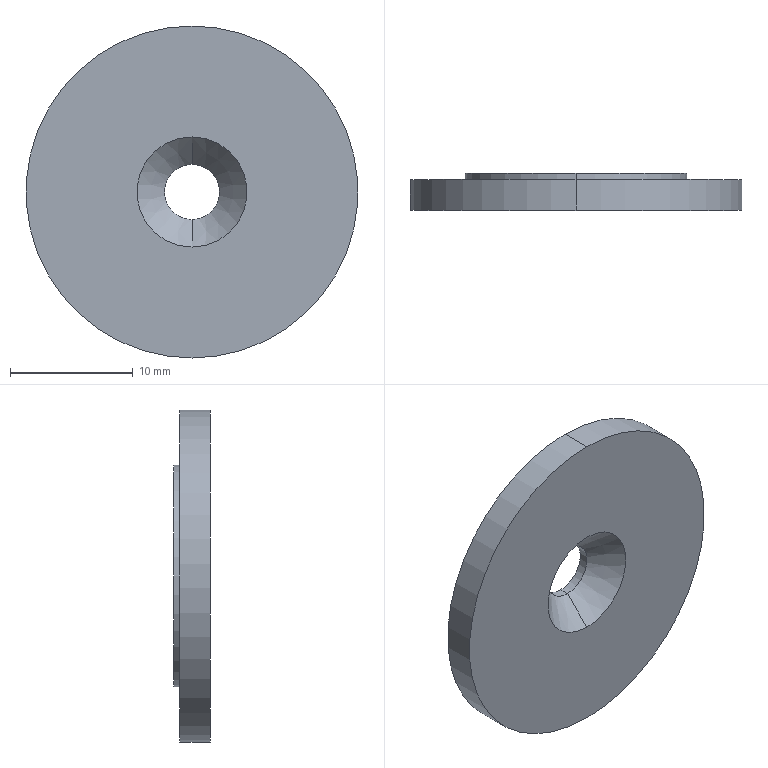Part | STEP file | ND25021-01-JDKM-14-TL | 1 solid | 11 faces | box 27 x 3 x 27 mm | volume 1464 mm3 | cylinder 6 | plane 3 | cone 2 | commonest cylinder face diameters 4.5 x2 18 x2 27 x2
STEP:
#1=CARTESIAN_POINT('',(0.,0.,0.));
#2=DIRECTION('',(0.,0.,1.));
#3=DIRECTION('',(1.,0.,0.));
#4=AXIS2_PLACEMENT_3D('',#1,#2,#3);
#5=CARTESIAN_POINT('',(0.,2.23,-2.25));
#6=VERTEX_POINT('',#5);
#7=CARTESIAN_POINT('',(0.,0.,-4.48));
#8=VERTEX_POINT('',#7);
#9=CARTESIAN_POINT('',(0.,0.,-4.48));
#10=DIRECTION('',(0.,-0.7071,-0.7071));
#11=VECTOR('',#10,1.);
#12=LINE('',#9,#11);
#13=CARTESIAN_POINT('',(0.,0.,0.));
#14=DIRECTION('',(0.,-1.,0.));
#15=DIRECTION('',(0.,0.,-1.));
#16=AXIS2_PLACEMENT_3D('',#13,#14,#15);
#17=CONICAL_SURFACE('',#16,4.48,0.7854);
#18=CARTESIAN_POINT('',(6.283,0.));
#19=DIRECTION('',(0.,1.));
#20=VECTOR('',#19,1.);
#21=LINE('',#18,#20);
#22=(GEOMETRIC_REPRESENTATION_CONTEXT(2)PARAMETRIC_REPRESENTATION_CONTEXT()REPRESENTATION_CONTEXT('',''));
#23=DEFINITIONAL_REPRESENTATION('',(#21),#22);
#24=PCURVE('',#17,#23);
#25=CARTESIAN_POINT('',(0.,0.,0.));
#26=DIRECTION('',(0.,-1.,0.));
#27=DIRECTION('',(0.,0.,-1.));
#28=AXIS2_PLACEMENT_3D('',#25,#26,#27);
#29=CONICAL_SURFACE('',#28,4.48,0.7854);
#30=CARTESIAN_POINT('',(0.,0.));
#31=DIRECTION('',(0.,1.));
#32=VECTOR('',#31,1.);
#33=LINE('',#30,#32);
#34=(GEOMETRIC_REPRESENTATION_CONTEXT(2)PARAMETRIC_REPRESENTATION_CONTEXT()REPRESENTATION_CONTEXT('',''));
#35=DEFINITIONAL_REPRESENTATION('',(#33),#34);
#36=PCURVE('',#29,#35);
#37=SURFACE_CURVE('',#12,(#24,#36),.PCURVE_S1.);
#38=EDGE_CURVE('',#6,#8,#37,.T.);
#39=ORIENTED_EDGE('',*,*,#38,.T.);
#40=CARTESIAN_POINT('',(0.,0.,4.48));
#41=VERTEX_POINT('',#40);
#42=CARTESIAN_POINT('',(0.,0.,0.));
#43=DIRECTION('',(0.,-1.,0.));
#44=DIRECTION('',(0.,0.,-1.));
#45=AXIS2_PLACEMENT_3D('',#42,#43,#44);
#46=CIRCLE('',#45,4.48);
#47=CARTESIAN_POINT('',(0.,0.));
#48=DIRECTION('',(1.,0.));
#49=VECTOR('',#48,1.);
#50=LINE('',#47,#49);
#51=(GEOMETRIC_REPRESENTATION_CONTEXT(2)PARAMETRIC_REPRESENTATION_CONTEXT()REPRESENTATION_CONTEXT('',''));
#52=DEFINITIONAL_REPRESENTATION('',(#50),#51);
#53=PCURVE('',#17,#52);
#54=CARTESIAN_POINT('',(0.,0.,0.));
#55=DIRECTION('',(0.,1.,0.));
#56=DIRECTION('',(0.,0.,1.));
#57=AXIS2_PLACEMENT_3D('',#54,#55,#56);
#58=PLANE('',#57);
#59=CARTESIAN_POINT('',(-4.48,0.));
#60=CARTESIAN_POINT('',(-4.48,7.76));
#61=CARTESIAN_POINT('',(2.24,3.88));
#62=CARTESIAN_POINT('',(8.96,0.));
#63=CARTESIAN_POINT('',(2.24,-3.88));
#64=CARTESIAN_POINT('',(-4.48,-7.76));
#65=CARTESIAN_POINT('',(-4.48,0.));
#66=(BOUNDED_CURVE()B_SPLINE_CURVE(2,(#59,#60,#61,#62,#63,#64,#65),.UNSPECIFIED.,.T.,.F.)B_SPLINE_CURVE_WITH_KNOTS((1,2,2,2,2,1),(-2.094,0.,2.094,4.189,6.283,8.378),.UNSPECIFIED.)CURVE()GEOMETRIC_REPRESENTATION_ITEM()RATIONAL_B_SPLINE_CURVE((1.,0.5,1.,0.5,1.,0.5,1.))REPRESENTATION_ITEM(''));
#67=(GEOMETRIC_REPRESENTATION_CONTEXT(2)PARAMETRIC_REPRESENTATION_CONTEXT()REPRESENTATION_CONTEXT('',''));
#68=DEFINITIONAL_REPRESENTATION('',(#66),#67);
#69=PCURVE('',#58,#68);
#70=SURFACE_CURVE('',#46,(#53,#69),.PCURVE_S1.);
#71=EDGE_CURVE('',#41,#8,#70,.T.);
#72=ORIENTED_EDGE('',*,*,#71,.F.);
#73=CARTESIAN_POINT('',(0.,2.23,2.25));
#74=VERTEX_POINT('',#73);
#75=CARTESIAN_POINT('',(0.,0.,4.48));
#76=DIRECTION('',(0.,-0.7071,0.7071));
#77=VECTOR('',#76,1.);
#78=LINE('',#75,#77);
#79=CARTESIAN_POINT('',(3.142,0.));
#80=DIRECTION('',(0.,1.));
#81=VECTOR('',#80,1.);
#82=LINE('',#79,#81);
#83=(GEOMETRIC_REPRESENTATION_CONTEXT(2)PARAMETRIC_REPRESENTATION_CONTEXT()REPRESENTATION_CONTEXT('',''));
#84=DEFINITIONAL_REPRESENTATION('',(#82),#83);
#85=PCURVE('',#17,#84);
#86=CARTESIAN_POINT('',(3.142,0.));
#87=DIRECTION('',(0.,1.));
#88=VECTOR('',#87,1.);
#89=LINE('',#86,#88);
#90=(GEOMETRIC_REPRESENTATION_CONTEXT(2)PARAMETRIC_REPRESENTATION_CONTEXT()REPRESENTATION_CONTEXT('',''));
#91=DEFINITIONAL_REPRESENTATION('',(#89),#90);
#92=PCURVE('',#29,#91);
#93=SURFACE_CURVE('',#78,(#85,#92),.PCURVE_S1.);
#94=EDGE_CURVE('',#74,#41,#93,.T.);
#95=ORIENTED_EDGE('',*,*,#94,.F.);
#96=CARTESIAN_POINT('',(0.,2.23,0.));
#97=DIRECTION('',(0.,-1.,0.));
#98=DIRECTION('',(0.,0.,-1.));
#99=AXIS2_PLACEMENT_3D('',#96,#97,#98);
#100=CIRCLE('',#99,2.25);
#101=CARTESIAN_POINT('',(0.,-2.23));
#102=DIRECTION('',(1.,0.));
#103=VECTOR('',#102,1.);
#104=LINE('',#101,#103);
#105=(GEOMETRIC_REPRESENTATION_CONTEXT(2)PARAMETRIC_REPRESENTATION_CONTEXT()REPRESENTATION_CONTEXT('',''));
#106=DEFINITIONAL_REPRESENTATION('',(#104),#105);
#107=PCURVE('',#17,#106);
#108=CARTESIAN_POINT('',(0.,0.,0.));
#109=DIRECTION('',(0.,-1.,0.));
#110=DIRECTION('',(0.,0.,-1.));
#111=AXIS2_PLACEMENT_3D('',#108,#109,#110);
#112=CYLINDRICAL_SURFACE('',#111,2.25);
#113=CARTESIAN_POINT('',(0.,-2.23));
#114=DIRECTION('',(1.,0.));
#115=VECTOR('',#114,1.);
#116=LINE('',#113,#115);
#117=(GEOMETRIC_REPRESENTATION_CONTEXT(2)PARAMETRIC_REPRESENTATION_CONTEXT()REPRESENTATION_CONTEXT('',''));
#118=DEFINITIONAL_REPRESENTATION('',(#116),#117);
#119=PCURVE('',#112,#118);
#120=SURFACE_CURVE('',#100,(#107,#119),.PCURVE_S1.);
#121=EDGE_CURVE('',#74,#6,#120,.T.);
#122=ORIENTED_EDGE('',*,*,#121,.T.);
#123=EDGE_LOOP('',(#39,#72,#95,#122));
#124=FACE_BOUND('',#123,.F.);
#125=ADVANCED_FACE('',(#124),#17,.F.);
#126=CARTESIAN_POINT('',(0.,3.,-2.25));
#127=VERTEX_POINT('',#126);
#128=CARTESIAN_POINT('',(0.,0.,-2.25));
#129=DIRECTION('',(0.,-1.,0.));
#130=VECTOR('',#129,1.);
#131=LINE('',#128,#130);
#132=CARTESIAN_POINT('',(6.283,0.));
#133=DIRECTION('',(0.,1.));
#134=VECTOR('',#133,1.);
#135=LINE('',#132,#134);
#136=(GEOMETRIC_REPRESENTATION_CONTEXT(2)PARAMETRIC_REPRESENTATION_CONTEXT()REPRESENTATION_CONTEXT('',''));
#137=DEFINITIONAL_REPRESENTATION('',(#135),#136);
#138=PCURVE('',#112,#137);
#139=CARTESIAN_POINT('',(0.,0.,0.));
#140=DIRECTION('',(0.,-1.,0.));
#141=DIRECTION('',(0.,0.,-1.));
#142=AXIS2_PLACEMENT_3D('',#139,#140,#141);
#143=CYLINDRICAL_SURFACE('',#142,2.25);
#144=CARTESIAN_POINT('',(0.,0.));
#145=DIRECTION('',(0.,1.));
#146=VECTOR('',#145,1.);
#147=LINE('',#144,#146);
#148=(GEOMETRIC_REPRESENTATION_CONTEXT(2)PARAMETRIC_REPRESENTATION_CONTEXT()REPRESENTATION_CONTEXT('',''));
#149=DEFINITIONAL_REPRESENTATION('',(#147),#148);
#150=PCURVE('',#143,#149);
#151=SURFACE_CURVE('',#131,(#138,#150),.PCURVE_S1.);
#152=EDGE_CURVE('',#127,#6,#151,.T.);
#153=ORIENTED_EDGE('',*,*,#152,.T.);
#154=ORIENTED_EDGE('',*,*,#121,.F.);
#155=CARTESIAN_POINT('',(0.,3.,2.25));
#156=VERTEX_POINT('',#155);
#157=CARTESIAN_POINT('',(0.,0.,2.25));
#158=DIRECTION('',(0.,-1.,0.));
#159=VECTOR('',#158,1.);
#160=LINE('',#157,#159);
#161=CARTESIAN_POINT('',(3.142,0.));
#162=DIRECTION('',(0.,1.));
#163=VECTOR('',#162,1.);
#164=LINE('',#161,#163);
#165=(GEOMETRIC_REPRESENTATION_CONTEXT(2)PARAMETRIC_REPRESENTATION_CONTEXT()REPRESENTATION_CONTEXT('',''));
#166=DEFINITIONAL_REPRESENTATION('',(#164),#165);
#167=PCURVE('',#112,#166);
#168=CARTESIAN_POINT('',(3.142,0.));
#169=DIRECTION('',(0.,1.));
#170=VECTOR('',#169,1.);
#171=LINE('',#168,#170);
#172=(GEOMETRIC_REPRESENTATION_CONTEXT(2)PARAMETRIC_REPRESENTATION_CONTEXT()REPRESENTATION_CONTEXT('',''));
#173=DEFINITIONAL_REPRESENTATION('',(#171),#172);
#174=PCURVE('',#143,#173);
#175=SURFACE_CURVE('',#160,(#167,#174),.PCURVE_S1.);
#176=EDGE_CURVE('',#156,#74,#175,.T.);
#177=ORIENTED_EDGE('',*,*,#176,.F.);
#178=CARTESIAN_POINT('',(0.,3.,0.));
#179=DIRECTION('',(0.,1.,0.));
#180=DIRECTION('',(0.,0.,1.));
#181=AXIS2_PLACEMENT_3D('',#178,#179,#180);
#182=CIRCLE('',#181,2.25);
#183=CARTESIAN_POINT('',(9.425,-3.));
#184=DIRECTION('',(-1.,0.));
#185=VECTOR('',#184,1.);
#186=LINE('',#183,#185);
#187=(GEOMETRIC_REPRESENTATION_CONTEXT(2)PARAMETRIC_REPRESENTATION_CONTEXT()REPRESENTATION_CONTEXT('',''));
#188=DEFINITIONAL_REPRESENTATION('',(#186),#187);
#189=PCURVE('',#112,#188);
#190=CARTESIAN_POINT('',(0.,3.,0.));
#191=DIRECTION('',(0.,1.,0.));
#192=DIRECTION('',(0.,0.,1.));
#193=AXIS2_PLACEMENT_3D('',#190,#191,#192);
#194=PLANE('',#193);
#195=CARTESIAN_POINT('',(0.,0.));
#196=DIRECTION('',(1.,0.));
#197=AXIS2_PLACEMENT_2D('',#195,#196);
#198=CIRCLE('',#197,2.25);
#199=(GEOMETRIC_REPRESENTATION_CONTEXT(2)PARAMETRIC_REPRESENTATION_CONTEXT()REPRESENTATION_CONTEXT('',''));
#200=DEFINITIONAL_REPRESENTATION('',(#198),#199);
#201=PCURVE('',#194,#200);
#202=SURFACE_CURVE('',#182,(#189,#201),.PCURVE_S1.);
#203=EDGE_CURVE('',#127,#156,#202,.T.);
#204=ORIENTED_EDGE('',*,*,#203,.F.);
#205=EDGE_LOOP('',(#153,#154,#177,#204));
#206=FACE_BOUND('',#205,.F.);
#207=ADVANCED_FACE('',(#206),#112,.F.);
#208=CARTESIAN_POINT('',(0.,3.,9.));
#209=VERTEX_POINT('',#208);
#210=CARTESIAN_POINT('',(0.,3.,-9.));
#211=VERTEX_POINT('',#210);
#212=CARTESIAN_POINT('',(0.,3.,0.));
#213=DIRECTION('',(0.,1.,0.));
#214=DIRECTION('',(0.,0.,1.));
#215=AXIS2_PLACEMENT_3D('',#212,#213,#214);
#216=CIRCLE('',#215,9.);
#217=CARTESIAN_POINT('',(0.,3.,0.));
#218=DIRECTION('',(0.,-1.,0.));
#219=DIRECTION('',(0.,0.,-1.));
#220=AXIS2_PLACEMENT_3D('',#217,#218,#219);
#221=CYLINDRICAL_SURFACE('',#220,9.);
#222=CARTESIAN_POINT('',(3.142,0.));
#223=DIRECTION('',(-1.,0.));
#224=VECTOR('',#223,1.);
#225=LINE('',#222,#224);
#226=(GEOMETRIC_REPRESENTATION_CONTEXT(2)PARAMETRIC_REPRESENTATION_CONTEXT()REPRESENTATION_CONTEXT('',''));
#227=DEFINITIONAL_REPRESENTATION('',(#225),#226);
#228=PCURVE('',#221,#227);
#229=CARTESIAN_POINT('',(0.,0.));
#230=DIRECTION('',(1.,0.));
#231=AXIS2_PLACEMENT_2D('',#229,#230);
#232=CIRCLE('',#231,9.);
#233=(GEOMETRIC_REPRESENTATION_CONTEXT(2)PARAMETRIC_REPRESENTATION_CONTEXT()REPRESENTATION_CONTEXT('',''));
#234=DEFINITIONAL_REPRESENTATION('',(#232),#233);
#235=PCURVE('',#194,#234);
#236=SURFACE_CURVE('',#216,(#228,#235),.PCURVE_S1.);
#237=EDGE_CURVE('',#209,#211,#236,.T.);
#238=ORIENTED_EDGE('',*,*,#237,.F.);
#239=CARTESIAN_POINT('',(0.,2.5,9.));
#240=VERTEX_POINT('',#239);
#241=CARTESIAN_POINT('',(0.,3.,9.));
#242=DIRECTION('',(0.,-1.,0.));
#243=VECTOR('',#242,1.);
#244=LINE('',#241,#243);
#245=CARTESIAN_POINT('',(3.142,0.));
#246=DIRECTION('',(0.,1.));
#247=VECTOR('',#246,1.);
#248=LINE('',#245,#247);
#249=(GEOMETRIC_REPRESENTATION_CONTEXT(2)PARAMETRIC_REPRESENTATION_CONTEXT()REPRESENTATION_CONTEXT('',''));
#250=DEFINITIONAL_REPRESENTATION('',(#248),#249);
#251=PCURVE('',#221,#250);
#252=CARTESIAN_POINT('',(0.,3.,0.));
#253=DIRECTION('',(0.,-1.,0.));
#254=DIRECTION('',(0.,0.,-1.));
#255=AXIS2_PLACEMENT_3D('',#252,#253,#254);
#256=CYLINDRICAL_SURFACE('',#255,9.);
#257=CARTESIAN_POINT('',(3.142,0.));
#258=DIRECTION('',(0.,1.));
#259=VECTOR('',#258,1.);
#260=LINE('',#257,#259);
#261=(GEOMETRIC_REPRESENTATION_CONTEXT(2)PARAMETRIC_REPRESENTATION_CONTEXT()REPRESENTATION_CONTEXT('',''));
#262=DEFINITIONAL_REPRESENTATION('',(#260),#261);
#263=PCURVE('',#256,#262);
#264=SURFACE_CURVE('',#244,(#251,#263),.PCURVE_S1.);
#265=EDGE_CURVE('',#209,#240,#264,.T.);
#266=ORIENTED_EDGE('',*,*,#265,.T.);
#267=CARTESIAN_POINT('',(0.,2.5,-9.));
#268=VERTEX_POINT('',#267);
#269=CARTESIAN_POINT('',(0.,2.5,0.));
#270=DIRECTION('',(0.,1.,0.));
#271=DIRECTION('',(0.,0.,1.));
#272=AXIS2_PLACEMENT_3D('',#269,#270,#271);
#273=CIRCLE('',#272,9.);
#274=CARTESIAN_POINT('',(3.142,0.5));
#275=DIRECTION('',(-1.,0.));
#276=VECTOR('',#275,1.);
#277=LINE('',#274,#276);
#278=(GEOMETRIC_REPRESENTATION_CONTEXT(2)PARAMETRIC_REPRESENTATION_CONTEXT()REPRESENTATION_CONTEXT('',''));
#279=DEFINITIONAL_REPRESENTATION('',(#277),#278);
#280=PCURVE('',#221,#279);
#281=CARTESIAN_POINT('',(0.,2.5,0.));
#282=DIRECTION('',(0.,1.,0.));
#283=DIRECTION('',(0.,0.,1.));
#284=AXIS2_PLACEMENT_3D('',#281,#282,#283);
#285=PLANE('',#284);
#286=CARTESIAN_POINT('',(0.,0.));
#287=DIRECTION('',(1.,0.));
#288=AXIS2_PLACEMENT_2D('',#286,#287);
#289=CIRCLE('',#288,9.);
#290=(GEOMETRIC_REPRESENTATION_CONTEXT(2)PARAMETRIC_REPRESENTATION_CONTEXT()REPRESENTATION_CONTEXT('',''));
#291=DEFINITIONAL_REPRESENTATION('',(#289),#290);
#292=PCURVE('',#285,#291);
#293=SURFACE_CURVE('',#273,(#280,#292),.PCURVE_S1.);
#294=EDGE_CURVE('',#240,#268,#293,.T.);
#295=ORIENTED_EDGE('',*,*,#294,.T.);
#296=CARTESIAN_POINT('',(0.,3.,-9.));
#297=DIRECTION('',(0.,-1.,0.));
#298=VECTOR('',#297,1.);
#299=LINE('',#296,#298);
#300=CARTESIAN_POINT('',(0.,0.));
#301=DIRECTION('',(0.,1.));
#302=VECTOR('',#301,1.);
#303=LINE('',#300,#302);
#304=(GEOMETRIC_REPRESENTATION_CONTEXT(2)PARAMETRIC_REPRESENTATION_CONTEXT()REPRESENTATION_CONTEXT('',''));
#305=DEFINITIONAL_REPRESENTATION('',(#303),#304);
#306=PCURVE('',#221,#305);
#307=CARTESIAN_POINT('',(6.283,0.));
#308=DIRECTION('',(0.,1.));
#309=VECTOR('',#308,1.);
#310=LINE('',#307,#309);
#311=(GEOMETRIC_REPRESENTATION_CONTEXT(2)PARAMETRIC_REPRESENTATION_CONTEXT()REPRESENTATION_CONTEXT('',''));
#312=DEFINITIONAL_REPRESENTATION('',(#310),#311);
#313=PCURVE('',#256,#312);
#314=SURFACE_CURVE('',#299,(#306,#313),.PCURVE_S1.);
#315=EDGE_CURVE('',#211,#268,#314,.T.);
#316=ORIENTED_EDGE('',*,*,#315,.F.);
#317=EDGE_LOOP('',(#238,#266,#295,#316));
#318=FACE_BOUND('',#317,.T.);
#319=ADVANCED_FACE('',(#318),#221,.T.);
#320=CARTESIAN_POINT('',(0.,2.5,13.5));
#321=VERTEX_POINT('',#320);
#322=CARTESIAN_POINT('',(0.,2.5,-13.5));
#323=VERTEX_POINT('',#322);
#324=CARTESIAN_POINT('',(0.,2.5,0.));
#325=DIRECTION('',(0.,1.,0.));
#326=DIRECTION('',(0.,0.,1.));
#327=AXIS2_PLACEMENT_3D('',#324,#325,#326);
#328=CIRCLE('',#327,13.5);
#329=CARTESIAN_POINT('',(0.,2.5,0.));
#330=DIRECTION('',(0.,-1.,0.));
#331=DIRECTION('',(0.,0.,-1.));
#332=AXIS2_PLACEMENT_3D('',#329,#330,#331);
#333=CYLINDRICAL_SURFACE('',#332,13.5);
#334=CARTESIAN_POINT('',(3.142,0.));
#335=DIRECTION('',(-1.,0.));
#336=VECTOR('',#335,1.);
#337=LINE('',#334,#336);
#338=(GEOMETRIC_REPRESENTATION_CONTEXT(2)PARAMETRIC_REPRESENTATION_CONTEXT()REPRESENTATION_CONTEXT('',''));
#339=DEFINITIONAL_REPRESENTATION('',(#337),#338);
#340=PCURVE('',#333,#339);
#341=CARTESIAN_POINT('',(0.,0.));
#342=DIRECTION('',(1.,0.));
#343=AXIS2_PLACEMENT_2D('',#341,#342);
#344=CIRCLE('',#343,13.5);
#345=(GEOMETRIC_REPRESENTATION_CONTEXT(2)PARAMETRIC_REPRESENTATION_CONTEXT()REPRESENTATION_CONTEXT('',''));
#346=DEFINITIONAL_REPRESENTATION('',(#344),#345);
#347=PCURVE('',#285,#346);
#348=SURFACE_CURVE('',#328,(#340,#347),.PCURVE_S1.);
#349=EDGE_CURVE('',#321,#323,#348,.T.);
#350=ORIENTED_EDGE('',*,*,#349,.F.);
#351=CARTESIAN_POINT('',(0.,0.,13.5));
#352=VERTEX_POINT('',#351);
#353=CARTESIAN_POINT('',(0.,2.5,13.5));
#354=DIRECTION('',(0.,-1.,0.));
#355=VECTOR('',#354,1.);
#356=LINE('',#353,#355);
#357=CARTESIAN_POINT('',(3.142,0.));
#358=DIRECTION('',(0.,1.));
#359=VECTOR('',#358,1.);
#360=LINE('',#357,#359);
#361=(GEOMETRIC_REPRESENTATION_CONTEXT(2)PARAMETRIC_REPRESENTATION_CONTEXT()REPRESENTATION_CONTEXT('',''));
#362=DEFINITIONAL_REPRESENTATION('',(#360),#361);
#363=PCURVE('',#333,#362);
#364=CARTESIAN_POINT('',(0.,2.5,0.));
#365=DIRECTION('',(0.,-1.,0.));
#366=DIRECTION('',(0.,0.,-1.));
#367=AXIS2_PLACEMENT_3D('',#364,#365,#366);
#368=CYLINDRICAL_SURFACE('',#367,13.5);
#369=CARTESIAN_POINT('',(3.142,0.));
#370=DIRECTION('',(0.,1.));
#371=VECTOR('',#370,1.);
#372=LINE('',#369,#371);
#373=(GEOMETRIC_REPRESENTATION_CONTEXT(2)PARAMETRIC_REPRESENTATION_CONTEXT()REPRESENTATION_CONTEXT('',''));
#374=DEFINITIONAL_REPRESENTATION('',(#372),#373);
#375=PCURVE('',#368,#374);
#376=SURFACE_CURVE('',#356,(#363,#375),.PCURVE_S1.);
#377=EDGE_CURVE('',#321,#352,#376,.T.);
#378=ORIENTED_EDGE('',*,*,#377,.T.);
#379=CARTESIAN_POINT('',(0.,0.,-13.5));
#380=VERTEX_POINT('',#379);
#381=CARTESIAN_POINT('',(0.,0.,0.));
#382=DIRECTION('',(0.,1.,0.));
#383=DIRECTION('',(0.,0.,1.));
#384=AXIS2_PLACEMENT_3D('',#381,#382,#383);
#385=CIRCLE('',#384,13.5);
#386=CARTESIAN_POINT('',(3.142,2.5));
#387=DIRECTION('',(-1.,0.));
#388=VECTOR('',#387,1.);
#389=LINE('',#386,#388);
#390=(GEOMETRIC_REPRESENTATION_CONTEXT(2)PARAMETRIC_REPRESENTATION_CONTEXT()REPRESENTATION_CONTEXT('',''));
#391=DEFINITIONAL_REPRESENTATION('',(#389),#390);
#392=PCURVE('',#333,#391);
#393=CARTESIAN_POINT('',(0.,0.));
#394=DIRECTION('',(1.,0.));
#395=AXIS2_PLACEMENT_2D('',#393,#394);
#396=CIRCLE('',#395,13.5);
#397=(GEOMETRIC_REPRESENTATION_CONTEXT(2)PARAMETRIC_REPRESENTATION_CONTEXT()REPRESENTATION_CONTEXT('',''));
#398=DEFINITIONAL_REPRESENTATION('',(#396),#397);
#399=PCURVE('',#58,#398);
#400=SURFACE_CURVE('',#385,(#392,#399),.PCURVE_S1.);
#401=EDGE_CURVE('',#352,#380,#400,.T.);
#402=ORIENTED_EDGE('',*,*,#401,.T.);
#403=CARTESIAN_POINT('',(0.,2.5,-13.5));
#404=DIRECTION('',(0.,-1.,0.));
#405=VECTOR('',#404,1.);
#406=LINE('',#403,#405);
#407=CARTESIAN_POINT('',(0.,0.));
#408=DIRECTION('',(0.,1.));
#409=VECTOR('',#408,1.);
#410=LINE('',#407,#409);
#411=(GEOMETRIC_REPRESENTATION_CONTEXT(2)PARAMETRIC_REPRESENTATION_CONTEXT()REPRESENTATION_CONTEXT('',''));
#412=DEFINITIONAL_REPRESENTATION('',(#410),#411);
#413=PCURVE('',#333,#412);
#414=CARTESIAN_POINT('',(6.283,0.));
#415=DIRECTION('',(0.,1.));
#416=VECTOR('',#415,1.);
#417=LINE('',#414,#416);
#418=(GEOMETRIC_REPRESENTATION_CONTEXT(2)PARAMETRIC_REPRESENTATION_CONTEXT()REPRESENTATION_CONTEXT('',''));
#419=DEFINITIONAL_REPRESENTATION('',(#417),#418);
#420=PCURVE('',#368,#419);
#421=SURFACE_CURVE('',#406,(#413,#420),.PCURVE_S1.);
#422=EDGE_CURVE('',#323,#380,#421,.T.);
#423=ORIENTED_EDGE('',*,*,#422,.F.);
#424=EDGE_LOOP('',(#350,#378,#402,#423));
#425=FACE_BOUND('',#424,.T.);
#426=ADVANCED_FACE('',(#425),#333,.T.);
#427=ORIENTED_EDGE('',*,*,#377,.F.);
#428=CARTESIAN_POINT('',(0.,2.5,0.));
#429=DIRECTION('',(0.,1.,0.));
#430=DIRECTION('',(0.,0.,1.));
#431=AXIS2_PLACEMENT_3D('',#428,#429,#430);
#432=CIRCLE('',#431,13.5);
#433=CARTESIAN_POINT('',(9.425,0.));
#434=DIRECTION('',(-1.,0.));
#435=VECTOR('',#434,1.);
#436=LINE('',#433,#435);
#437=(GEOMETRIC_REPRESENTATION_CONTEXT(2)PARAMETRIC_REPRESENTATION_CONTEXT()REPRESENTATION_CONTEXT('',''));
#438=DEFINITIONAL_REPRESENTATION('',(#436),#437);
#439=PCURVE('',#368,#438);
#440=CARTESIAN_POINT('',(0.,0.));
#441=DIRECTION('',(1.,0.));
#442=AXIS2_PLACEMENT_2D('',#440,#441);
#443=CIRCLE('',#442,13.5);
#444=(GEOMETRIC_REPRESENTATION_CONTEXT(2)PARAMETRIC_REPRESENTATION_CONTEXT()REPRESENTATION_CONTEXT('',''));
#445=DEFINITIONAL_REPRESENTATION('',(#443),#444);
#446=PCURVE('',#285,#445);
#447=SURFACE_CURVE('',#432,(#439,#446),.PCURVE_S1.);
#448=EDGE_CURVE('',#323,#321,#447,.T.);
#449=ORIENTED_EDGE('',*,*,#448,.F.);
#450=ORIENTED_EDGE('',*,*,#422,.T.);
#451=CARTESIAN_POINT('',(0.,0.,0.));
#452=DIRECTION('',(0.,1.,0.));
#453=DIRECTION('',(0.,0.,1.));
#454=AXIS2_PLACEMENT_3D('',#451,#452,#453);
#455=CIRCLE('',#454,13.5);
#456=CARTESIAN_POINT('',(9.425,2.5));
#457=DIRECTION('',(-1.,0.));
#458=VECTOR('',#457,1.);
#459=LINE('',#456,#458);
#460=(GEOMETRIC_REPRESENTATION_CONTEXT(2)PARAMETRIC_REPRESENTATION_CONTEXT()REPRESENTATION_CONTEXT('',''));
#461=DEFINITIONAL_REPRESENTATION('',(#459),#460);
#462=PCURVE('',#368,#461);
#463=CARTESIAN_POINT('',(0.,0.));
#464=DIRECTION('',(1.,0.));
#465=AXIS2_PLACEMENT_2D('',#463,#464);
#466=CIRCLE('',#465,13.5);
#467=(GEOMETRIC_REPRESENTATION_CONTEXT(2)PARAMETRIC_REPRESENTATION_CONTEXT()REPRESENTATION_CONTEXT('',''));
#468=DEFINITIONAL_REPRESENTATION('',(#466),#467);
#469=PCURVE('',#58,#468);
#470=SURFACE_CURVE('',#455,(#462,#469),.PCURVE_S1.);
#471=EDGE_CURVE('',#380,#352,#470,.T.);
#472=ORIENTED_EDGE('',*,*,#471,.T.);
#473=EDGE_LOOP('',(#427,#449,#450,#472));
#474=FACE_BOUND('',#473,.T.);
#475=ADVANCED_FACE('',(#474),#368,.T.);
#476=CARTESIAN_POINT('',(0.,2.5,0.));
#477=DIRECTION('',(0.,1.,0.));
#478=DIRECTION('',(0.,0.,1.));
#479=AXIS2_PLACEMENT_3D('',#476,#477,#478);
#480=CIRCLE('',#479,9.);
#481=CARTESIAN_POINT('',(0.,0.));
#482=DIRECTION('',(1.,0.));
#483=AXIS2_PLACEMENT_2D('',#481,#482);
#484=CIRCLE('',#483,9.);
#485=(GEOMETRIC_REPRESENTATION_CONTEXT(2)PARAMETRIC_REPRESENTATION_CONTEXT()REPRESENTATION_CONTEXT('',''));
#486=DEFINITIONAL_REPRESENTATION('',(#484),#485);
#487=PCURVE('',#285,#486);
#488=CARTESIAN_POINT('',(9.425,0.5));
#489=DIRECTION('',(-1.,0.));
#490=VECTOR('',#489,1.);
#491=LINE('',#488,#490);
#492=(GEOMETRIC_REPRESENTATION_CONTEXT(2)PARAMETRIC_REPRESENTATION_CONTEXT()REPRESENTATION_CONTEXT('',''));
#493=DEFINITIONAL_REPRESENTATION('',(#491),#492);
#494=PCURVE('',#256,#493);
#495=SURFACE_CURVE('',#480,(#487,#494),.PCURVE_S1.);
#496=EDGE_CURVE('',#268,#240,#495,.T.);
#497=ORIENTED_EDGE('',*,*,#496,.F.);
#498=ORIENTED_EDGE('',*,*,#294,.F.);
#499=EDGE_LOOP('',(#497,#498));
#500=FACE_BOUND('',#499,.T.);
#501=ORIENTED_EDGE('',*,*,#448,.T.);
#502=ORIENTED_EDGE('',*,*,#349,.T.);
#503=EDGE_LOOP('',(#501,#502));
#504=FACE_BOUND('',#503,.T.);
#505=ADVANCED_FACE('',(#500,#504),#285,.T.);
#506=CARTESIAN_POINT('',(0.,0.,0.));
#507=DIRECTION('',(0.,-1.,0.));
#508=DIRECTION('',(0.,0.,-1.));
#509=AXIS2_PLACEMENT_3D('',#506,#507,#508);
#510=CIRCLE('',#509,4.48);
#511=CARTESIAN_POINT('',(-4.48,0.));
#512=CARTESIAN_POINT('',(-4.48,7.76));
#513=CARTESIAN_POINT('',(2.24,3.88));
#514=CARTESIAN_POINT('',(8.96,0.));
#515=CARTESIAN_POINT('',(2.24,-3.88));
#516=CARTESIAN_POINT('',(-4.48,-7.76));
#517=CARTESIAN_POINT('',(-4.48,0.));
#518=(BOUNDED_CURVE()B_SPLINE_CURVE(2,(#511,#512,#513,#514,#515,#516,#517),.UNSPECIFIED.,.T.,.F.)B_SPLINE_CURVE_WITH_KNOTS((1,2,2,2,2,1),(-2.094,0.,2.094,4.189,6.283,8.378),.UNSPECIFIED.)CURVE()GEOMETRIC_REPRESENTATION_ITEM()RATIONAL_B_SPLINE_CURVE((1.,0.5,1.,0.5,1.,0.5,1.))REPRESENTATION_ITEM(''));
#519=(GEOMETRIC_REPRESENTATION_CONTEXT(2)PARAMETRIC_REPRESENTATION_CONTEXT()REPRESENTATION_CONTEXT('',''));
#520=DEFINITIONAL_REPRESENTATION('',(#518),#519);
#521=PCURVE('',#58,#520);
#522=CARTESIAN_POINT('',(0.,0.));
#523=DIRECTION('',(1.,0.));
#524=VECTOR('',#523,1.);
#525=LINE('',#522,#524);
#526=(GEOMETRIC_REPRESENTATION_CONTEXT(2)PARAMETRIC_REPRESENTATION_CONTEXT()REPRESENTATION_CONTEXT('',''));
#527=DEFINITIONAL_REPRESENTATION('',(#525),#526);
#528=PCURVE('',#29,#527);
#529=SURFACE_CURVE('',#510,(#521,#528),.PCURVE_S1.);
#530=EDGE_CURVE('',#8,#41,#529,.T.);
#531=ORIENTED_EDGE('',*,*,#530,.F.);
#532=ORIENTED_EDGE('',*,*,#71,.F.);
#533=EDGE_LOOP('',(#531,#532));
#534=FACE_BOUND('',#533,.T.);
#535=ORIENTED_EDGE('',*,*,#471,.F.);
#536=ORIENTED_EDGE('',*,*,#401,.F.);
#537=EDGE_LOOP('',(#535,#536));
#538=FACE_BOUND('',#537,.T.);
#539=ADVANCED_FACE('',(#534,#538),#58,.F.);
#540=ORIENTED_EDGE('',*,*,#265,.F.);
#541=CARTESIAN_POINT('',(0.,3.,0.));
#542=DIRECTION('',(0.,1.,0.));
#543=DIRECTION('',(0.,0.,1.));
#544=AXIS2_PLACEMENT_3D('',#541,#542,#543);
#545=CIRCLE('',#544,9.);
#546=CARTESIAN_POINT('',(9.425,0.));
#547=DIRECTION('',(-1.,0.));
#548=VECTOR('',#547,1.);
#549=LINE('',#546,#548);
#550=(GEOMETRIC_REPRESENTATION_CONTEXT(2)PARAMETRIC_REPRESENTATION_CONTEXT()REPRESENTATION_CONTEXT('',''));
#551=DEFINITIONAL_REPRESENTATION('',(#549),#550);
#552=PCURVE('',#256,#551);
#553=CARTESIAN_POINT('',(0.,0.));
#554=DIRECTION('',(1.,0.));
#555=AXIS2_PLACEMENT_2D('',#553,#554);
#556=CIRCLE('',#555,9.);
#557=(GEOMETRIC_REPRESENTATION_CONTEXT(2)PARAMETRIC_REPRESENTATION_CONTEXT()REPRESENTATION_CONTEXT('',''));
#558=DEFINITIONAL_REPRESENTATION('',(#556),#557);
#559=PCURVE('',#194,#558);
#560=SURFACE_CURVE('',#545,(#552,#559),.PCURVE_S1.);
#561=EDGE_CURVE('',#211,#209,#560,.T.);
#562=ORIENTED_EDGE('',*,*,#561,.F.);
#563=ORIENTED_EDGE('',*,*,#315,.T.);
#564=ORIENTED_EDGE('',*,*,#496,.T.);
#565=EDGE_LOOP('',(#540,#562,#563,#564));
#566=FACE_BOUND('',#565,.T.);
#567=ADVANCED_FACE('',(#566),#256,.T.);
#568=ORIENTED_EDGE('',*,*,#203,.F.);
#569=CARTESIAN_POINT('',(0.,3.,0.));
#570=DIRECTION('',(0.,1.,0.));
#571=DIRECTION('',(0.,0.,1.));
#572=AXIS2_PLACEMENT_3D('',#569,#570,#571);
#573=CIRCLE('',#572,2.25);
#574=CARTESIAN_POINT('',(0.,0.));
#575=DIRECTION('',(1.,0.));
#576=AXIS2_PLACEMENT_2D('',#574,#575);
#577=CIRCLE('',#576,2.25);
#578=(GEOMETRIC_REPRESENTATION_CONTEXT(2)PARAMETRIC_REPRESENTATION_CONTEXT()REPRESENTATION_CONTEXT('',''));
#579=DEFINITIONAL_REPRESENTATION('',(#577),#578);
#580=PCURVE('',#194,#579);
#581=CARTESIAN_POINT('',(3.142,-3.));
#582=DIRECTION('',(-1.,0.));
#583=VECTOR('',#582,1.);
#584=LINE('',#581,#583);
#585=(GEOMETRIC_REPRESENTATION_CONTEXT(2)PARAMETRIC_REPRESENTATION_CONTEXT()REPRESENTATION_CONTEXT('',''));
#586=DEFINITIONAL_REPRESENTATION('',(#584),#585);
#587=PCURVE('',#143,#586);
#588=SURFACE_CURVE('',#573,(#580,#587),.PCURVE_S1.);
#589=EDGE_CURVE('',#156,#127,#588,.T.);
#590=ORIENTED_EDGE('',*,*,#589,.F.);
#591=EDGE_LOOP('',(#568,#590));
#592=FACE_BOUND('',#591,.T.);
#593=ORIENTED_EDGE('',*,*,#561,.T.);
#594=ORIENTED_EDGE('',*,*,#237,.T.);
#595=EDGE_LOOP('',(#593,#594));
#596=FACE_BOUND('',#595,.T.);
#597=ADVANCED_FACE('',(#592,#596),#194,.T.);
#598=CARTESIAN_POINT('',(0.,2.23,0.));
#599=DIRECTION('',(0.,-1.,0.));
#600=DIRECTION('',(0.,0.,-1.));
#601=AXIS2_PLACEMENT_3D('',#598,#599,#600);
#602=CIRCLE('',#601,2.25);
#603=CARTESIAN_POINT('',(0.,-2.23));
#604=DIRECTION('',(1.,0.));
#605=VECTOR('',#604,1.);
#606=LINE('',#603,#605);
#607=(GEOMETRIC_REPRESENTATION_CONTEXT(2)PARAMETRIC_REPRESENTATION_CONTEXT()REPRESENTATION_CONTEXT('',''));
#608=DEFINITIONAL_REPRESENTATION('',(#606),#607);
#609=PCURVE('',#143,#608);
#610=CARTESIAN_POINT('',(0.,-2.23));
#611=DIRECTION('',(1.,0.));
#612=VECTOR('',#611,1.);
#613=LINE('',#610,#612);
#614=(GEOMETRIC_REPRESENTATION_CONTEXT(2)PARAMETRIC_REPRESENTATION_CONTEXT()REPRESENTATION_CONTEXT('',''));
#615=DEFINITIONAL_REPRESENTATION('',(#613),#614);
#616=PCURVE('',#29,#615);
#617=SURFACE_CURVE('',#602,(#609,#616),.PCURVE_S1.);
#618=EDGE_CURVE('',#6,#74,#617,.T.);
#619=ORIENTED_EDGE('',*,*,#618,.F.);
#620=ORIENTED_EDGE('',*,*,#152,.F.);
#621=ORIENTED_EDGE('',*,*,#589,.F.);
#622=ORIENTED_EDGE('',*,*,#176,.T.);
#623=EDGE_LOOP('',(#619,#620,#621,#622));
#624=FACE_BOUND('',#623,.F.);
#625=ADVANCED_FACE('',(#624),#143,.F.);
#626=ORIENTED_EDGE('',*,*,#530,.F.);
#627=ORIENTED_EDGE('',*,*,#38,.F.);
#628=ORIENTED_EDGE('',*,*,#618,.T.);
#629=ORIENTED_EDGE('',*,*,#94,.T.);
#630=EDGE_LOOP('',(#626,#627,#628,#629));
#631=FACE_BOUND('',#630,.F.);
#632=ADVANCED_FACE('',(#631),#29,.F.);
#633=CLOSED_SHELL('',(#125,#207,#319,#426,#475,#505,#539,#567,#597,#625,#632));
#634=MANIFOLD_SOLID_BREP('',#633);
#635=(LENGTH_UNIT()NAMED_UNIT(*)SI_UNIT(.MILLI.,.METRE.));
#636=UNCERTAINTY_MEASURE_WITH_UNIT(LENGTH_MEASURE(0.0000001),#635,'','');
#637=(NAMED_UNIT(*)PLANE_ANGLE_UNIT()SI_UNIT($,.RADIAN.));
#638=(NAMED_UNIT(*)SI_UNIT($,.STERADIAN.)SOLID_ANGLE_UNIT());
#639=(GEOMETRIC_REPRESENTATION_CONTEXT(3)GLOBAL_UNCERTAINTY_ASSIGNED_CONTEXT((#636))GLOBAL_UNIT_ASSIGNED_CONTEXT((#635,#637,#638))REPRESENTATION_CONTEXT('',''));
#640=ADVANCED_BREP_SHAPE_REPRESENTATION('',(#4,#634),#639);